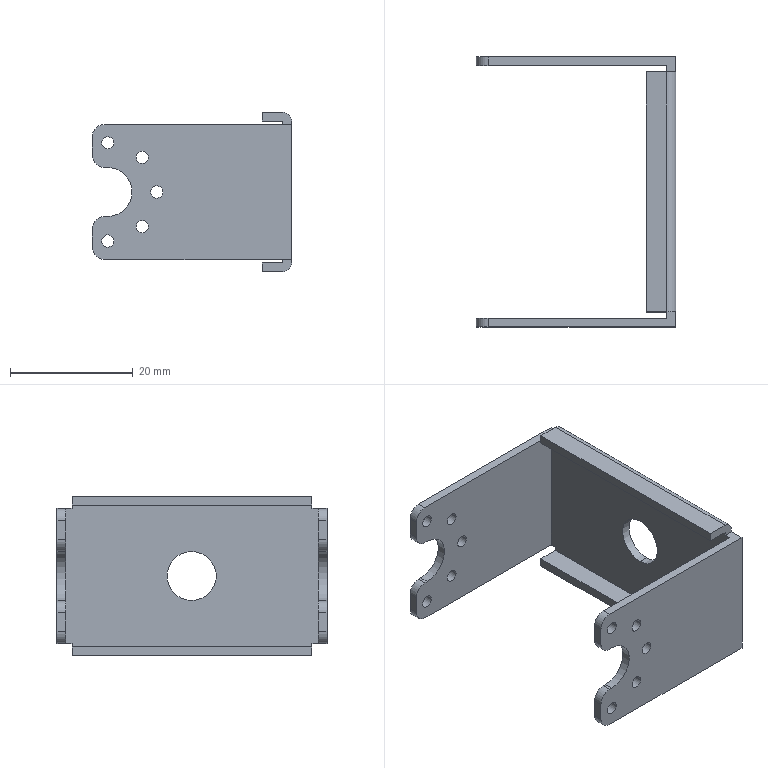Part | SolidWorks | features BaseBody 1 | 1 solid | 66 faces | box 32.495 x 44 x 26 mm | volume 3696 mm3 | cylinder 34 | plane 32 | commonest cylinder face diameters 2 x20 4 x8 8 x4 2.9 x2